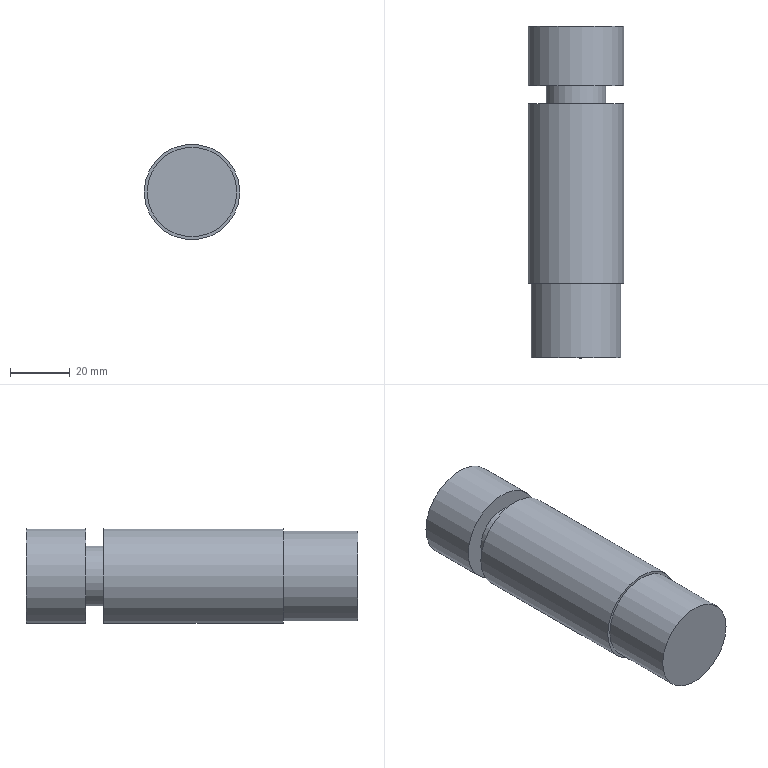Part | NX | features solid 2 | 1 solid | 9 faces | box 32 x 111 x 32 mm | volume 83896 mm3 | plane 5 | cylinder 4 | commonest cylinder face diameters 32 x2 20 x1 30 x1
STEP:
#1=CARTESIAN_POINT('',(-146.,155.,210.));
#2=VERTEX_POINT('',#1);
#3=CARTESIAN_POINT('',(-130.,155.,210.));
#4=DIRECTION('',(0.,1.,0.));
#5=DIRECTION('',(-1.,0.,0.));
#6=AXIS2_PLACEMENT_3D('',#3,#4,#5);
#7=CIRCLE('',#6,16.);
#8=EDGE_CURVE('',#2,#2,#7,.T.);
#9=ORIENTED_EDGE('',*,*,#8,.T.);
#10=EDGE_LOOP('',(#9));
#11=FACE_BOUND('',#10,.T.);
#12=CARTESIAN_POINT('',(-140.,155.,210.));
#13=VERTEX_POINT('',#12);
#14=CARTESIAN_POINT('',(-130.,155.,210.));
#15=DIRECTION('',(0.,1.,0.));
#16=DIRECTION('',(-1.,0.,0.));
#17=AXIS2_PLACEMENT_3D('',#14,#15,#16);
#18=CIRCLE('',#17,10.);
#19=EDGE_CURVE('',#13,#13,#18,.T.);
#20=ORIENTED_EDGE('',*,*,#19,.F.);
#21=EDGE_LOOP('',(#20));
#22=FACE_BOUND('',#21,.T.);
#23=CARTESIAN_POINT('',(-130.,155.,210.));
#24=DIRECTION('',(0.,1.,0.));
#25=DIRECTION('',(0.,0.,-1.));
#26=AXIS2_PLACEMENT_3D('',#23,#24,#25);
#27=PLANE('',#26);
#28=ADVANCED_FACE('',(#11,#22),#27,.T.);
#29=ORIENTED_EDGE('',*,*,#8,.F.);
#30=EDGE_LOOP('',(#29));
#31=FACE_BOUND('',#30,.T.);
#32=CARTESIAN_POINT('',(-146.,95.,210.));
#33=VERTEX_POINT('',#32);
#34=CARTESIAN_POINT('',(-130.,95.,210.));
#35=DIRECTION('',(0.,1.,0.));
#36=DIRECTION('',(-1.,0.,0.));
#37=AXIS2_PLACEMENT_3D('',#34,#35,#36);
#38=CIRCLE('',#37,16.);
#39=EDGE_CURVE('',#33,#33,#38,.T.);
#40=ORIENTED_EDGE('',*,*,#39,.T.);
#41=EDGE_LOOP('',(#40));
#42=FACE_BOUND('',#41,.T.);
#43=CARTESIAN_POINT('',(-130.,155.,210.));
#44=DIRECTION('',(0.,-1.,0.));
#45=DIRECTION('',(0.,0.,1.));
#46=AXIS2_PLACEMENT_3D('',#43,#44,#45);
#47=CYLINDRICAL_SURFACE('',#46,16.);
#48=ADVANCED_FACE('',(#31,#42),#47,.T.);
#49=CARTESIAN_POINT('',(-145.,95.,210.));
#50=VERTEX_POINT('',#49);
#51=CARTESIAN_POINT('',(-130.,95.,210.));
#52=DIRECTION('',(0.,1.,0.));
#53=DIRECTION('',(-1.,0.,0.));
#54=AXIS2_PLACEMENT_3D('',#51,#52,#53);
#55=CIRCLE('',#54,15.);
#56=EDGE_CURVE('',#50,#50,#55,.T.);
#57=ORIENTED_EDGE('',*,*,#56,.T.);
#58=EDGE_LOOP('',(#57));
#59=FACE_BOUND('',#58,.T.);
#60=ORIENTED_EDGE('',*,*,#39,.F.);
#61=EDGE_LOOP('',(#60));
#62=FACE_BOUND('',#61,.T.);
#63=CARTESIAN_POINT('',(-130.,95.,210.));
#64=DIRECTION('',(0.,1.,0.));
#65=DIRECTION('',(0.,0.,-1.));
#66=AXIS2_PLACEMENT_3D('',#63,#64,#65);
#67=PLANE('',#66);
#68=ADVANCED_FACE('',(#59,#62),#67,.F.);
#69=CARTESIAN_POINT('',(-145.,70.,210.));
#70=VERTEX_POINT('',#69);
#71=CARTESIAN_POINT('',(-130.,70.,210.));
#72=DIRECTION('',(0.,1.,0.));
#73=DIRECTION('',(-1.,0.,0.));
#74=AXIS2_PLACEMENT_3D('',#71,#72,#73);
#75=CIRCLE('',#74,15.);
#76=EDGE_CURVE('',#70,#70,#75,.T.);
#77=ORIENTED_EDGE('',*,*,#76,.T.);
#78=EDGE_LOOP('',(#77));
#79=FACE_BOUND('',#78,.T.);
#80=ORIENTED_EDGE('',*,*,#56,.F.);
#81=EDGE_LOOP('',(#80));
#82=FACE_BOUND('',#81,.T.);
#83=CARTESIAN_POINT('',(-130.,70.,210.));
#84=DIRECTION('',(0.,1.,0.));
#85=DIRECTION('',(0.,0.,-1.));
#86=AXIS2_PLACEMENT_3D('',#83,#84,#85);
#87=CYLINDRICAL_SURFACE('',#86,15.);
#88=ADVANCED_FACE('',(#79,#82),#87,.T.);
#89=ORIENTED_EDGE('',*,*,#76,.F.);
#90=EDGE_LOOP('',(#89));
#91=FACE_BOUND('',#90,.T.);
#92=CARTESIAN_POINT('',(-130.,70.,210.));
#93=DIRECTION('',(0.,1.,0.));
#94=DIRECTION('',(0.,0.,-1.));
#95=AXIS2_PLACEMENT_3D('',#92,#93,#94);
#96=PLANE('',#95);
#97=ADVANCED_FACE('',(#91),#96,.F.);
#98=CARTESIAN_POINT('',(-140.,161.,210.));
#99=VERTEX_POINT('',#98);
#100=CARTESIAN_POINT('',(-130.,161.,210.));
#101=DIRECTION('',(0.,1.,0.));
#102=DIRECTION('',(-1.,0.,0.));
#103=AXIS2_PLACEMENT_3D('',#100,#101,#102);
#104=CIRCLE('',#103,10.);
#105=EDGE_CURVE('',#99,#99,#104,.T.);
#106=ORIENTED_EDGE('',*,*,#105,.F.);
#107=EDGE_LOOP('',(#106));
#108=FACE_BOUND('',#107,.T.);
#109=ORIENTED_EDGE('',*,*,#19,.T.);
#110=EDGE_LOOP('',(#109));
#111=FACE_BOUND('',#110,.T.);
#112=CARTESIAN_POINT('',(-130.,161.,210.));
#113=DIRECTION('',(0.,-1.,0.));
#114=DIRECTION('',(0.,0.,1.));
#115=AXIS2_PLACEMENT_3D('',#112,#113,#114);
#116=CYLINDRICAL_SURFACE('',#115,10.);
#117=ADVANCED_FACE('',(#108,#111),#116,.T.);
#118=CARTESIAN_POINT('',(-146.,161.,210.));
#119=VERTEX_POINT('',#118);
#120=CARTESIAN_POINT('',(-130.,161.,210.));
#121=DIRECTION('',(0.,1.,0.));
#122=DIRECTION('',(-1.,0.,0.));
#123=AXIS2_PLACEMENT_3D('',#120,#121,#122);
#124=CIRCLE('',#123,16.);
#125=EDGE_CURVE('',#119,#119,#124,.T.);
#126=ORIENTED_EDGE('',*,*,#125,.F.);
#127=EDGE_LOOP('',(#126));
#128=FACE_BOUND('',#127,.T.);
#129=ORIENTED_EDGE('',*,*,#105,.T.);
#130=EDGE_LOOP('',(#129));
#131=FACE_BOUND('',#130,.T.);
#132=CARTESIAN_POINT('',(-130.,161.,210.));
#133=DIRECTION('',(0.,1.,0.));
#134=DIRECTION('',(0.,0.,-1.));
#135=AXIS2_PLACEMENT_3D('',#132,#133,#134);
#136=PLANE('',#135);
#137=ADVANCED_FACE('',(#128,#131),#136,.F.);
#138=CARTESIAN_POINT('',(-146.,181.,210.));
#139=VERTEX_POINT('',#138);
#140=CARTESIAN_POINT('',(-130.,181.,210.));
#141=DIRECTION('',(0.,1.,0.));
#142=DIRECTION('',(-1.,0.,0.));
#143=AXIS2_PLACEMENT_3D('',#140,#141,#142);
#144=CIRCLE('',#143,16.);
#145=EDGE_CURVE('',#139,#139,#144,.T.);
#146=ORIENTED_EDGE('',*,*,#145,.F.);
#147=EDGE_LOOP('',(#146));
#148=FACE_BOUND('',#147,.T.);
#149=ORIENTED_EDGE('',*,*,#125,.T.);
#150=EDGE_LOOP('',(#149));
#151=FACE_BOUND('',#150,.T.);
#152=CARTESIAN_POINT('',(-130.,181.,210.));
#153=DIRECTION('',(0.,-1.,0.));
#154=DIRECTION('',(0.,0.,1.));
#155=AXIS2_PLACEMENT_3D('',#152,#153,#154);
#156=CYLINDRICAL_SURFACE('',#155,16.);
#157=ADVANCED_FACE('',(#148,#151),#156,.T.);
#158=ORIENTED_EDGE('',*,*,#145,.T.);
#159=EDGE_LOOP('',(#158));
#160=FACE_BOUND('',#159,.T.);
#161=CARTESIAN_POINT('',(-130.,181.,210.));
#162=DIRECTION('',(0.,1.,0.));
#163=DIRECTION('',(0.,0.,-1.));
#164=AXIS2_PLACEMENT_3D('',#161,#162,#163);
#165=PLANE('',#164);
#166=ADVANCED_FACE('',(#160),#165,.T.);
#167=CLOSED_SHELL('',(#28,#48,#68,#88,#97,#117,#137,#157,#166));
#168=MANIFOLD_SOLID_BREP('',#167);
#169=(LENGTH_UNIT()NAMED_UNIT(*)SI_UNIT(.MILLI.,.METRE.));
#170=UNCERTAINTY_MEASURE_WITH_UNIT(LENGTH_MEASURE(0.00001),#169,'','');
#171=(NAMED_UNIT(*)PLANE_ANGLE_UNIT()SI_UNIT($,.RADIAN.));
#172=(NAMED_UNIT(*)SI_UNIT($,.STERADIAN.)SOLID_ANGLE_UNIT());
#173=(GEOMETRIC_REPRESENTATION_CONTEXT(3)GLOBAL_UNCERTAINTY_ASSIGNED_CONTEXT((#170))GLOBAL_UNIT_ASSIGNED_CONTEXT((#169,#171,#172))REPRESENTATION_CONTEXT('',''));
#174=ADVANCED_BREP_SHAPE_REPRESENTATION('',(#168),#173);